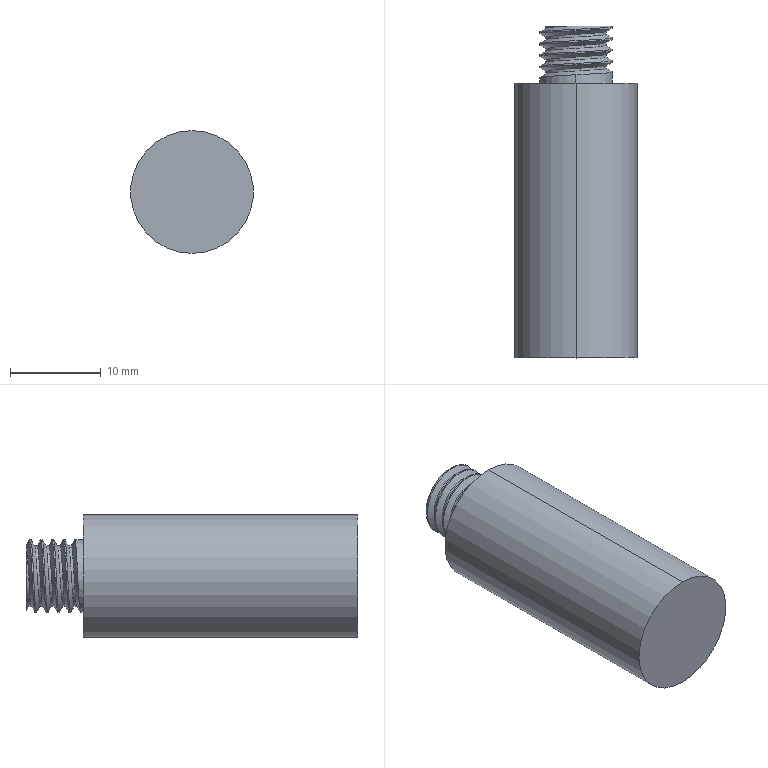Part | SolidWorks | features BaseBody 1 | 1 solid | 23 faces | box 13.5 x 36.5 x 13.5 mm | volume 4034 mm3 | cylinder 15 | plane 5 | spline 3 | commonest cylinder face diameters 8 x11 4.85 x2 13.5 x2